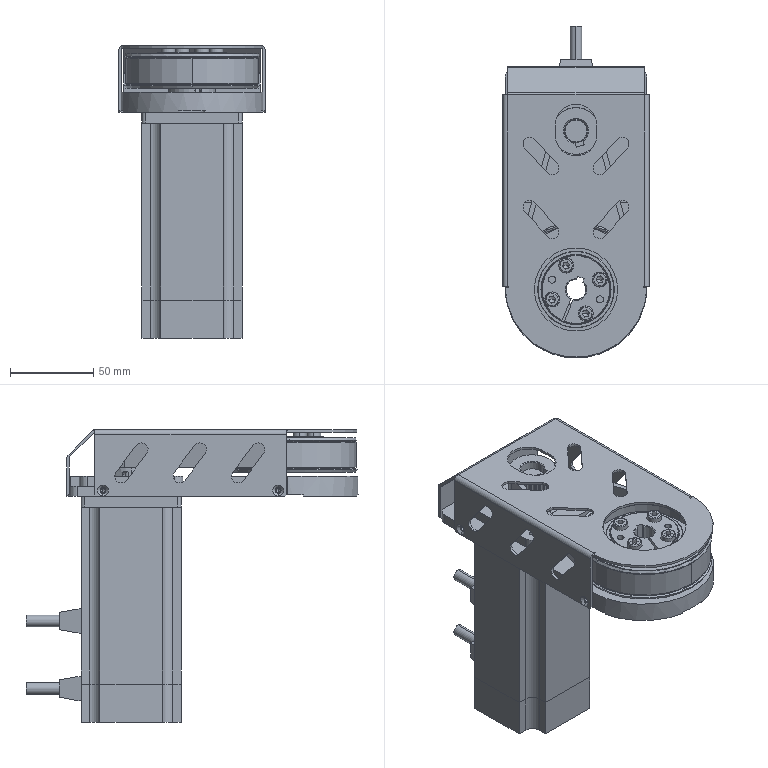Part | STEP file | Copy of CZ006-400W side link 3:1(K60)^K50A-1H20-S(formula driven)-L300-motor left- | 19 solids | 1174 faces | box 88 x 199.001 x 175.5 mm | volume 672015 mm3 | cylinder 784 | plane 262 | cone 110 | spline 18 | commonest cylinder face diameters 0.6 x269 1.82 x161 76.62 x82 8 x31 25.2 x28 5.5 x24